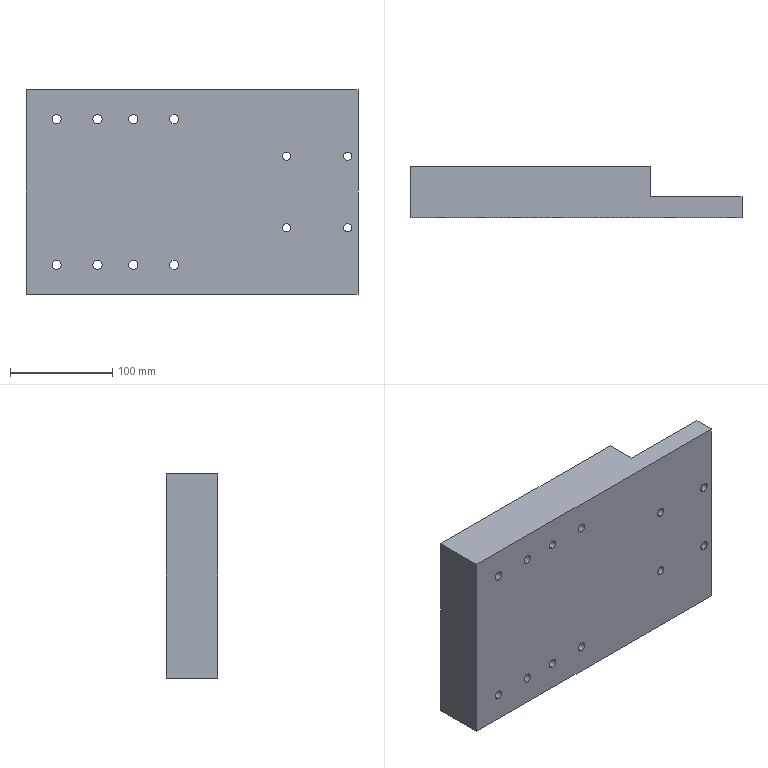Part | SolidWorks | features ICE 3, BaseBody 1 | 1 solid | 81 faces | box 325 x 50 x 200 mm | volume 2147505 mm3 | cylinder 48 | plane 25 | cone 8 | commonest cylinder face diameters 9 x24 15 x24